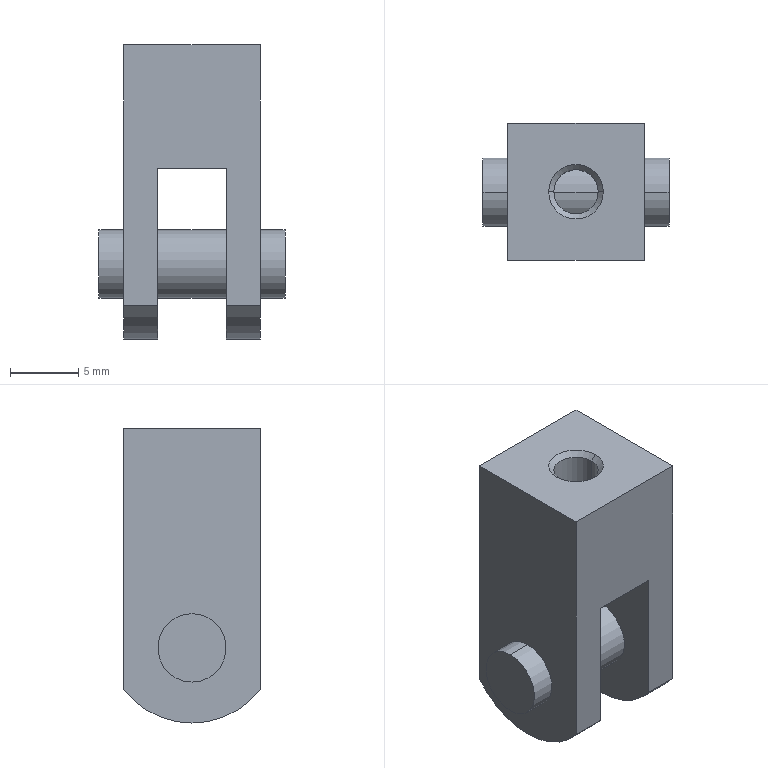Part | STEP file | Y_P010_Y-P010 | 1 solid | 22 faces | box 13.6 x 10 x 21.5 mm | volume 1582 mm3 | cylinder 10 | plane 10 | cone 2 | commonest cylinder face diameters 5 x6 3.24 x2 12.6 x2
STEP:
#1=CARTESIAN_POINT('',(6.8,0.,-18.5));
#2=VERTEX_POINT('',#1);
#3=CARTESIAN_POINT('',(6.8,0.,-13.5));
#4=VERTEX_POINT('',#3);
#5=CARTESIAN_POINT('',(6.8,0.,-16.));
#6=DIRECTION('',(1.,0.,0.));
#7=DIRECTION('',(0.,0.,-1.));
#8=AXIS2_PLACEMENT_3D('',#5,#6,#7);
#9=CIRCLE('',#8,2.5);
#10=EDGE_CURVE('',#2,#4,#9,.T.);
#11=ORIENTED_EDGE('',*,*,#10,.F.);
#12=CARTESIAN_POINT('',(5.,0.,-18.5));
#13=VERTEX_POINT('',#12);
#14=CARTESIAN_POINT('',(6.8,0.,-18.5));
#15=DIRECTION('',(-1.,0.,0.));
#16=VECTOR('',#15,1000.);
#17=LINE('',#14,#16);
#18=EDGE_CURVE('',#2,#13,#17,.T.);
#19=ORIENTED_EDGE('',*,*,#18,.T.);
#20=CARTESIAN_POINT('',(5.,0.,-13.5));
#21=VERTEX_POINT('',#20);
#22=CARTESIAN_POINT('',(5.,0.,-16.));
#23=DIRECTION('',(-1.,0.,0.));
#24=DIRECTION('',(0.,0.,-1.));
#25=AXIS2_PLACEMENT_3D('',#22,#23,#24);
#26=CIRCLE('',#25,2.5);
#27=EDGE_CURVE('',#21,#13,#26,.T.);
#28=ORIENTED_EDGE('',*,*,#27,.F.);
#29=CARTESIAN_POINT('',(6.8,0.,-13.5));
#30=DIRECTION('',(-1.,0.,0.));
#31=VECTOR('',#30,1000.);
#32=LINE('',#29,#31);
#33=EDGE_CURVE('',#4,#21,#32,.T.);
#34=ORIENTED_EDGE('',*,*,#33,.F.);
#35=EDGE_LOOP('',(#11,#19,#28,#34));
#36=FACE_OUTER_BOUND('',#35,.T.);
#37=CARTESIAN_POINT('',(6.8,0.,-16.));
#38=DIRECTION('',(-1.,0.,0.));
#39=DIRECTION('',(0.,0.,1.));
#40=AXIS2_PLACEMENT_3D('',#37,#38,#39);
#41=CYLINDRICAL_SURFACE('',#40,2.5);
#42=ADVANCED_FACE('',(#36),#41,.T.);
#43=CARTESIAN_POINT('',(-5.,0.,-13.5));
#44=VERTEX_POINT('',#43);
#45=CARTESIAN_POINT('',(-5.,0.,-18.5));
#46=VERTEX_POINT('',#45);
#47=CARTESIAN_POINT('',(-5.,0.,-16.));
#48=DIRECTION('',(-1.,0.,0.));
#49=DIRECTION('',(0.,0.,-1.));
#50=AXIS2_PLACEMENT_3D('',#47,#48,#49);
#51=CIRCLE('',#50,2.5);
#52=EDGE_CURVE('',#44,#46,#51,.T.);
#53=ORIENTED_EDGE('',*,*,#52,.T.);
#54=CARTESIAN_POINT('',(-6.8,0.,-18.5));
#55=VERTEX_POINT('',#54);
#56=CARTESIAN_POINT('',(6.8,0.,-18.5));
#57=DIRECTION('',(-1.,0.,0.));
#58=VECTOR('',#57,1000.);
#59=LINE('',#56,#58);
#60=EDGE_CURVE('',#46,#55,#59,.T.);
#61=ORIENTED_EDGE('',*,*,#60,.T.);
#62=CARTESIAN_POINT('',(-6.8,0.,-13.5));
#63=VERTEX_POINT('',#62);
#64=CARTESIAN_POINT('',(-6.8,0.,-16.));
#65=DIRECTION('',(1.,0.,0.));
#66=DIRECTION('',(0.,0.,-1.));
#67=AXIS2_PLACEMENT_3D('',#64,#65,#66);
#68=CIRCLE('',#67,2.5);
#69=EDGE_CURVE('',#55,#63,#68,.T.);
#70=ORIENTED_EDGE('',*,*,#69,.T.);
#71=CARTESIAN_POINT('',(6.8,0.,-13.5));
#72=DIRECTION('',(-1.,0.,0.));
#73=VECTOR('',#72,1000.);
#74=LINE('',#71,#73);
#75=EDGE_CURVE('',#44,#63,#74,.T.);
#76=ORIENTED_EDGE('',*,*,#75,.F.);
#77=EDGE_LOOP('',(#53,#61,#70,#76));
#78=FACE_OUTER_BOUND('',#77,.T.);
#79=CARTESIAN_POINT('',(6.8,0.,-16.));
#80=DIRECTION('',(-1.,0.,0.));
#81=DIRECTION('',(0.,0.,1.));
#82=AXIS2_PLACEMENT_3D('',#79,#80,#81);
#83=CYLINDRICAL_SURFACE('',#82,2.5);
#84=ADVANCED_FACE('',(#78),#83,.T.);
#85=CARTESIAN_POINT('',(2.5,0.,-13.5));
#86=VERTEX_POINT('',#85);
#87=CARTESIAN_POINT('',(2.5,0.,-18.5));
#88=VERTEX_POINT('',#87);
#89=CARTESIAN_POINT('',(2.5,0.,-16.));
#90=DIRECTION('',(-1.,0.,0.));
#91=DIRECTION('',(0.,0.,-1.));
#92=AXIS2_PLACEMENT_3D('',#89,#90,#91);
#93=CIRCLE('',#92,2.5);
#94=EDGE_CURVE('',#86,#88,#93,.T.);
#95=ORIENTED_EDGE('',*,*,#94,.T.);
#96=CARTESIAN_POINT('',(-2.5,0.,-18.5));
#97=VERTEX_POINT('',#96);
#98=CARTESIAN_POINT('',(6.8,0.,-18.5));
#99=DIRECTION('',(-1.,0.,0.));
#100=VECTOR('',#99,1000.);
#101=LINE('',#98,#100);
#102=EDGE_CURVE('',#88,#97,#101,.T.);
#103=ORIENTED_EDGE('',*,*,#102,.T.);
#104=CARTESIAN_POINT('',(-2.5,0.,-13.5));
#105=VERTEX_POINT('',#104);
#106=CARTESIAN_POINT('',(-2.5,0.,-16.));
#107=DIRECTION('',(-1.,0.,0.));
#108=DIRECTION('',(0.,0.,-1.));
#109=AXIS2_PLACEMENT_3D('',#106,#107,#108);
#110=CIRCLE('',#109,2.5);
#111=EDGE_CURVE('',#105,#97,#110,.T.);
#112=ORIENTED_EDGE('',*,*,#111,.F.);
#113=CARTESIAN_POINT('',(6.8,0.,-13.5));
#114=DIRECTION('',(-1.,0.,0.));
#115=VECTOR('',#114,1000.);
#116=LINE('',#113,#115);
#117=EDGE_CURVE('',#86,#105,#116,.T.);
#118=ORIENTED_EDGE('',*,*,#117,.F.);
#119=EDGE_LOOP('',(#95,#103,#112,#118));
#120=FACE_OUTER_BOUND('',#119,.T.);
#121=CARTESIAN_POINT('',(6.8,0.,-16.));
#122=DIRECTION('',(-1.,0.,0.));
#123=DIRECTION('',(0.,0.,1.));
#124=AXIS2_PLACEMENT_3D('',#121,#122,#123);
#125=CYLINDRICAL_SURFACE('',#124,2.5);
#126=ADVANCED_FACE('',(#120),#125,.T.);
#127=CARTESIAN_POINT('',(-1.62,0.,-9.));
#128=VERTEX_POINT('',#127);
#129=CARTESIAN_POINT('',(1.62,0.,-9.));
#130=VERTEX_POINT('',#129);
#131=CARTESIAN_POINT('',(0.,0.,-9.));
#132=DIRECTION('',(0.,0.,1.));
#133=DIRECTION('',(1.,0.,0.));
#134=AXIS2_PLACEMENT_3D('',#131,#132,#133);
#135=CIRCLE('',#134,1.62);
#136=EDGE_CURVE('',#128,#130,#135,.T.);
#137=ORIENTED_EDGE('',*,*,#136,.F.);
#138=CARTESIAN_POINT('',(-1.62,0.,-0.38));
#139=VERTEX_POINT('',#138);
#140=CARTESIAN_POINT('',(-1.62,0.,-9.));
#141=DIRECTION('',(0.,0.,1.));
#142=VECTOR('',#141,1000.);
#143=LINE('',#140,#142);
#144=EDGE_CURVE('',#128,#139,#143,.T.);
#145=ORIENTED_EDGE('',*,*,#144,.T.);
#146=CARTESIAN_POINT('',(1.62,0.,-0.38));
#147=VERTEX_POINT('',#146);
#148=CARTESIAN_POINT('',(0.,0.,-0.38));
#149=DIRECTION('',(0.,0.,1.));
#150=DIRECTION('',(1.,0.,0.));
#151=AXIS2_PLACEMENT_3D('',#148,#149,#150);
#152=CIRCLE('',#151,1.62);
#153=EDGE_CURVE('',#139,#147,#152,.T.);
#154=ORIENTED_EDGE('',*,*,#153,.T.);
#155=CARTESIAN_POINT('',(1.62,0.,-9.));
#156=DIRECTION('',(0.,0.,1.));
#157=VECTOR('',#156,1000.);
#158=LINE('',#155,#157);
#159=EDGE_CURVE('',#130,#147,#158,.T.);
#160=ORIENTED_EDGE('',*,*,#159,.F.);
#161=EDGE_LOOP('',(#137,#145,#154,#160));
#162=FACE_OUTER_BOUND('',#161,.T.);
#163=CARTESIAN_POINT('',(0.,0.,-9.));
#164=DIRECTION('',(0.,0.,1.));
#165=DIRECTION('',(1.,0.,0.));
#166=AXIS2_PLACEMENT_3D('',#163,#164,#165);
#167=CYLINDRICAL_SURFACE('',#166,1.62);
#168=ADVANCED_FACE('',(#162),#167,.F.);
#169=ORIENTED_EDGE('',*,*,#153,.F.);
#170=CARTESIAN_POINT('',(-2.,0.,0.));
#171=VERTEX_POINT('',#170);
#172=CARTESIAN_POINT('',(-1.62,0.,-0.38));
#173=DIRECTION('',(-0.7071,0.,0.7071));
#174=VECTOR('',#173,1000.);
#175=LINE('',#172,#174);
#176=EDGE_CURVE('',#139,#171,#175,.T.);
#177=ORIENTED_EDGE('',*,*,#176,.T.);
#178=CARTESIAN_POINT('',(2.,0.,0.));
#179=VERTEX_POINT('',#178);
#180=CARTESIAN_POINT('',(0.,0.,0.));
#181=DIRECTION('',(0.,0.,1.));
#182=DIRECTION('',(-1.,0.,0.));
#183=AXIS2_PLACEMENT_3D('',#180,#181,#182);
#184=CIRCLE('',#183,2.);
#185=EDGE_CURVE('',#171,#179,#184,.T.);
#186=ORIENTED_EDGE('',*,*,#185,.T.);
#187=CARTESIAN_POINT('',(1.62,0.,-0.38));
#188=DIRECTION('',(0.7071,0.,0.7071));
#189=VECTOR('',#188,1000.);
#190=LINE('',#187,#189);
#191=EDGE_CURVE('',#147,#179,#190,.T.);
#192=ORIENTED_EDGE('',*,*,#191,.F.);
#193=EDGE_LOOP('',(#169,#177,#186,#192));
#194=FACE_OUTER_BOUND('',#193,.T.);
#195=CARTESIAN_POINT('',(0.,0.,-0.38));
#196=DIRECTION('',(0.,0.,1.));
#197=DIRECTION('',(1.,0.,0.));
#198=AXIS2_PLACEMENT_3D('',#195,#196,#197);
#199=CONICAL_SURFACE('',#198,1.62,0.7854);
#200=ADVANCED_FACE('',(#194),#199,.F.);
#201=CARTESIAN_POINT('',(5.,5.,0.));
#202=VERTEX_POINT('',#201);
#203=CARTESIAN_POINT('',(5.,-5.,0.));
#204=VERTEX_POINT('',#203);
#205=CARTESIAN_POINT('',(5.,5.,0.));
#206=DIRECTION('',(0.,-1.,0.));
#207=VECTOR('',#206,1000.);
#208=LINE('',#205,#207);
#209=EDGE_CURVE('',#202,#204,#208,.T.);
#210=ORIENTED_EDGE('',*,*,#209,.T.);
#211=CARTESIAN_POINT('',(5.,-5.,-19.033));
#212=VERTEX_POINT('',#211);
#213=CARTESIAN_POINT('',(5.,-5.,0.));
#214=DIRECTION('',(0.,0.,-1.));
#215=VECTOR('',#214,1000.);
#216=LINE('',#213,#215);
#217=EDGE_CURVE('',#204,#212,#216,.T.);
#218=ORIENTED_EDGE('',*,*,#217,.T.);
#219=CARTESIAN_POINT('',(5.,5.,-19.033));
#220=VERTEX_POINT('',#219);
#221=CARTESIAN_POINT('',(5.,0.,-15.2));
#222=DIRECTION('',(1.,0.,0.));
#223=DIRECTION('',(0.,0.,-1.));
#224=AXIS2_PLACEMENT_3D('',#221,#222,#223);
#225=CIRCLE('',#224,6.3);
#226=EDGE_CURVE('',#212,#220,#225,.T.);
#227=ORIENTED_EDGE('',*,*,#226,.T.);
#228=CARTESIAN_POINT('',(5.,5.,-19.033));
#229=DIRECTION('',(0.,0.,1.));
#230=VECTOR('',#229,1000.);
#231=LINE('',#228,#230);
#232=EDGE_CURVE('',#220,#202,#231,.T.);
#233=ORIENTED_EDGE('',*,*,#232,.T.);
#234=EDGE_LOOP('',(#210,#218,#227,#233));
#235=FACE_OUTER_BOUND('',#234,.T.);
#236=ORIENTED_EDGE('',*,*,#27,.T.);
#237=CARTESIAN_POINT('',(5.,0.,-16.));
#238=DIRECTION('',(-1.,0.,0.));
#239=DIRECTION('',(0.,0.,-1.));
#240=AXIS2_PLACEMENT_3D('',#237,#238,#239);
#241=CIRCLE('',#240,2.5);
#242=EDGE_CURVE('',#13,#21,#241,.T.);
#243=ORIENTED_EDGE('',*,*,#242,.T.);
#244=EDGE_LOOP('',(#236,#243));
#245=FACE_BOUND('',#244,.T.);
#246=CARTESIAN_POINT('',(5.,0.,-15.2));
#247=DIRECTION('',(1.,0.,0.));
#248=DIRECTION('',(0.,0.,-1.));
#249=AXIS2_PLACEMENT_3D('',#246,#247,#248);
#250=PLANE('',#249);
#251=ADVANCED_FACE('',(#235,#245),#250,.T.);
#252=CARTESIAN_POINT('',(-5.,5.,0.));
#253=VERTEX_POINT('',#252);
#254=CARTESIAN_POINT('',(-5.,-5.,0.));
#255=VERTEX_POINT('',#254);
#256=CARTESIAN_POINT('',(-5.,5.,0.));
#257=DIRECTION('',(0.,-1.,0.));
#258=VECTOR('',#257,1000.);
#259=LINE('',#256,#258);
#260=EDGE_CURVE('',#253,#255,#259,.T.);
#261=ORIENTED_EDGE('',*,*,#260,.F.);
#262=CARTESIAN_POINT('',(-5.,5.,-19.033));
#263=VERTEX_POINT('',#262);
#264=CARTESIAN_POINT('',(-5.,5.,-19.033));
#265=DIRECTION('',(0.,0.,1.));
#266=VECTOR('',#265,1000.);
#267=LINE('',#264,#266);
#268=EDGE_CURVE('',#263,#253,#267,.T.);
#269=ORIENTED_EDGE('',*,*,#268,.F.);
#270=CARTESIAN_POINT('',(-5.,-5.,-19.033));
#271=VERTEX_POINT('',#270);
#272=CARTESIAN_POINT('',(-5.,0.,-15.2));
#273=DIRECTION('',(1.,0.,0.));
#274=DIRECTION('',(0.,0.,-1.));
#275=AXIS2_PLACEMENT_3D('',#272,#273,#274);
#276=CIRCLE('',#275,6.3);
#277=EDGE_CURVE('',#271,#263,#276,.T.);
#278=ORIENTED_EDGE('',*,*,#277,.F.);
#279=CARTESIAN_POINT('',(-5.,-5.,0.));
#280=DIRECTION('',(0.,0.,-1.));
#281=VECTOR('',#280,1000.);
#282=LINE('',#279,#281);
#283=EDGE_CURVE('',#255,#271,#282,.T.);
#284=ORIENTED_EDGE('',*,*,#283,.F.);
#285=EDGE_LOOP('',(#261,#269,#278,#284));
#286=FACE_OUTER_BOUND('',#285,.T.);
#287=ORIENTED_EDGE('',*,*,#52,.F.);
#288=CARTESIAN_POINT('',(-5.,0.,-16.));
#289=DIRECTION('',(-1.,0.,0.));
#290=DIRECTION('',(0.,0.,-1.));
#291=AXIS2_PLACEMENT_3D('',#288,#289,#290);
#292=CIRCLE('',#291,2.5);
#293=EDGE_CURVE('',#46,#44,#292,.T.);
#294=ORIENTED_EDGE('',*,*,#293,.F.);
#295=EDGE_LOOP('',(#287,#294));
#296=FACE_BOUND('',#295,.T.);
#297=CARTESIAN_POINT('',(-5.,0.,-15.2));
#298=DIRECTION('',(1.,0.,0.));
#299=DIRECTION('',(0.,0.,-1.));
#300=AXIS2_PLACEMENT_3D('',#297,#298,#299);
#301=PLANE('',#300);
#302=ADVANCED_FACE('',(#286,#296),#301,.F.);
#303=CARTESIAN_POINT('',(-2.5,-5.,-9.));
#304=VERTEX_POINT('',#303);
#305=CARTESIAN_POINT('',(-2.5,-5.,-19.033));
#306=VERTEX_POINT('',#305);
#307=CARTESIAN_POINT('',(-2.5,-5.,0.));
#308=DIRECTION('',(0.,0.,-1.));
#309=VECTOR('',#308,1000.);
#310=LINE('',#307,#309);
#311=EDGE_CURVE('',#304,#306,#310,.T.);
#312=ORIENTED_EDGE('',*,*,#311,.T.);
#313=CARTESIAN_POINT('',(-2.5,5.,-19.033));
#314=VERTEX_POINT('',#313);
#315=CARTESIAN_POINT('',(-2.5,0.,-15.2));
#316=DIRECTION('',(1.,0.,0.));
#317=DIRECTION('',(0.,0.,-1.));
#318=AXIS2_PLACEMENT_3D('',#315,#316,#317);
#319=CIRCLE('',#318,6.3);
#320=EDGE_CURVE('',#306,#314,#319,.T.);
#321=ORIENTED_EDGE('',*,*,#320,.T.);
#322=CARTESIAN_POINT('',(-2.5,5.,-9.));
#323=VERTEX_POINT('',#322);
#324=CARTESIAN_POINT('',(-2.5,5.,-19.033));
#325=DIRECTION('',(0.,0.,1.));
#326=VECTOR('',#325,1000.);
#327=LINE('',#324,#326);
#328=EDGE_CURVE('',#314,#323,#327,.T.);
#329=ORIENTED_EDGE('',*,*,#328,.T.);
#330=CARTESIAN_POINT('',(-2.5,5.01,-9.));
#331=DIRECTION('',(0.,-1.,0.));
#332=VECTOR('',#331,1000.);
#333=LINE('',#330,#332);
#334=EDGE_CURVE('',#323,#304,#333,.T.);
#335=ORIENTED_EDGE('',*,*,#334,.T.);
#336=EDGE_LOOP('',(#312,#321,#329,#335));
#337=FACE_OUTER_BOUND('',#336,.T.);
#338=ORIENTED_EDGE('',*,*,#111,.T.);
#339=CARTESIAN_POINT('',(-2.5,0.,-16.));
#340=DIRECTION('',(-1.,0.,0.));
#341=DIRECTION('',(0.,0.,-1.));
#342=AXIS2_PLACEMENT_3D('',#339,#340,#341);
#343=CIRCLE('',#342,2.5);
#344=EDGE_CURVE('',#97,#105,#343,.T.);
#345=ORIENTED_EDGE('',*,*,#344,.T.);
#346=EDGE_LOOP('',(#338,#345));
#347=FACE_BOUND('',#346,.T.);
#348=CARTESIAN_POINT('',(-2.5,-5.01,-9.));
#349=DIRECTION('',(1.,0.,0.));
#350=DIRECTION('',(0.,0.,-1.));
#351=AXIS2_PLACEMENT_3D('',#348,#349,#350);
#352=PLANE('',#351);
#353=ADVANCED_FACE('',(#337,#347),#352,.T.);
#354=CARTESIAN_POINT('',(2.5,5.,-9.));
#355=VERTEX_POINT('',#354);
#356=CARTESIAN_POINT('',(2.5,-5.,-9.));
#357=VERTEX_POINT('',#356);
#358=CARTESIAN_POINT('',(2.5,5.01,-9.));
#359=DIRECTION('',(0.,-1.,0.));
#360=VECTOR('',#359,1000.);
#361=LINE('',#358,#360);
#362=EDGE_CURVE('',#355,#357,#361,.T.);
#363=ORIENTED_EDGE('',*,*,#362,.F.);
#364=CARTESIAN_POINT('',(2.5,5.,-19.033));
#365=VERTEX_POINT('',#364);
#366=CARTESIAN_POINT('',(2.5,5.,-19.033));
#367=DIRECTION('',(0.,0.,1.));
#368=VECTOR('',#367,1000.);
#369=LINE('',#366,#368);
#370=EDGE_CURVE('',#365,#355,#369,.T.);
#371=ORIENTED_EDGE('',*,*,#370,.F.);
#372=CARTESIAN_POINT('',(2.5,-5.,-19.033));
#373=VERTEX_POINT('',#372);
#374=CARTESIAN_POINT('',(2.5,0.,-15.2));
#375=DIRECTION('',(1.,0.,0.));
#376=DIRECTION('',(0.,0.,-1.));
#377=AXIS2_PLACEMENT_3D('',#374,#375,#376);
#378=CIRCLE('',#377,6.3);
#379=EDGE_CURVE('',#373,#365,#378,.T.);
#380=ORIENTED_EDGE('',*,*,#379,.F.);
#381=CARTESIAN_POINT('',(2.5,-5.,0.));
#382=DIRECTION('',(0.,0.,-1.));
#383=VECTOR('',#382,1000.);
#384=LINE('',#381,#383);
#385=EDGE_CURVE('',#357,#373,#384,.T.);
#386=ORIENTED_EDGE('',*,*,#385,.F.);
#387=EDGE_LOOP('',(#363,#371,#380,#386));
#388=FACE_OUTER_BOUND('',#387,.T.);
#389=ORIENTED_EDGE('',*,*,#94,.F.);
#390=CARTESIAN_POINT('',(2.5,0.,-16.));
#391=DIRECTION('',(-1.,0.,0.));
#392=DIRECTION('',(0.,0.,-1.));
#393=AXIS2_PLACEMENT_3D('',#390,#391,#392);
#394=CIRCLE('',#393,2.5);
#395=EDGE_CURVE('',#88,#86,#394,.T.);
#396=ORIENTED_EDGE('',*,*,#395,.F.);
#397=EDGE_LOOP('',(#389,#396));
#398=FACE_BOUND('',#397,.T.);
#399=CARTESIAN_POINT('',(2.5,-5.01,-9.));
#400=DIRECTION('',(1.,0.,0.));
#401=DIRECTION('',(0.,0.,-1.));
#402=AXIS2_PLACEMENT_3D('',#399,#400,#401);
#403=PLANE('',#402);
#404=ADVANCED_FACE('',(#388,#398),#403,.F.);
#405=CARTESIAN_POINT('',(5.,5.,0.));
#406=DIRECTION('',(-1.,0.,0.));
#407=VECTOR('',#406,1000.);
#408=LINE('',#405,#407);
#409=EDGE_CURVE('',#202,#253,#408,.T.);
#410=ORIENTED_EDGE('',*,*,#409,.T.);
#411=ORIENTED_EDGE('',*,*,#260,.T.);
#412=CARTESIAN_POINT('',(5.,-5.,0.));
#413=DIRECTION('',(-1.,0.,0.));
#414=VECTOR('',#413,1000.);
#415=LINE('',#412,#414);
#416=EDGE_CURVE('',#204,#255,#415,.T.);
#417=ORIENTED_EDGE('',*,*,#416,.F.);
#418=ORIENTED_EDGE('',*,*,#209,.F.);
#419=EDGE_LOOP('',(#410,#411,#417,#418));
#420=FACE_OUTER_BOUND('',#419,.T.);
#421=CARTESIAN_POINT('',(0.,0.,0.));
#422=DIRECTION('',(0.,0.,1.));
#423=DIRECTION('',(-1.,0.,0.));
#424=AXIS2_PLACEMENT_3D('',#421,#422,#423);
#425=CIRCLE('',#424,2.);
#426=EDGE_CURVE('',#179,#171,#425,.T.);
#427=ORIENTED_EDGE('',*,*,#426,.F.);
#428=ORIENTED_EDGE('',*,*,#185,.F.);
#429=EDGE_LOOP('',(#427,#428));
#430=FACE_BOUND('',#429,.T.);
#431=CARTESIAN_POINT('',(5.,5.,0.));
#432=DIRECTION('',(0.,0.,-1.));
#433=DIRECTION('',(-1.,0.,0.));
#434=AXIS2_PLACEMENT_3D('',#431,#432,#433);
#435=PLANE('',#434);
#436=ADVANCED_FACE('',(#420,#430),#435,.F.);
#437=ORIENTED_EDGE('',*,*,#334,.F.);
#438=CARTESIAN_POINT('',(5.,5.,-9.));
#439=DIRECTION('',(-1.,0.,0.));
#440=VECTOR('',#439,1000.);
#441=LINE('',#438,#440);
#442=EDGE_CURVE('',#355,#323,#441,.T.);
#443=ORIENTED_EDGE('',*,*,#442,.F.);
#444=ORIENTED_EDGE('',*,*,#362,.T.);
#445=CARTESIAN_POINT('',(5.,-5.,-9.));
#446=DIRECTION('',(1.,0.,0.));
#447=VECTOR('',#446,1000.);
#448=LINE('',#445,#447);
#449=EDGE_CURVE('',#304,#357,#448,.T.);
#450=ORIENTED_EDGE('',*,*,#449,.F.);
#451=EDGE_LOOP('',(#437,#443,#444,#450));
#452=FACE_OUTER_BOUND('',#451,.T.);
#453=CARTESIAN_POINT('',(0.,0.,-9.));
#454=DIRECTION('',(0.,0.,1.));
#455=DIRECTION('',(1.,0.,0.));
#456=AXIS2_PLACEMENT_3D('',#453,#454,#455);
#457=CIRCLE('',#456,1.62);
#458=EDGE_CURVE('',#130,#128,#457,.T.);
#459=ORIENTED_EDGE('',*,*,#458,.T.);
#460=ORIENTED_EDGE('',*,*,#136,.T.);
#461=EDGE_LOOP('',(#459,#460));
#462=FACE_BOUND('',#461,.T.);
#463=CARTESIAN_POINT('',(-2.5,5.01,-9.));
#464=DIRECTION('',(0.,0.,1.));
#465=DIRECTION('',(1.,0.,0.));
#466=AXIS2_PLACEMENT_3D('',#463,#464,#465);
#467=PLANE('',#466);
#468=ADVANCED_FACE('',(#452,#462),#467,.F.);
#469=ORIENTED_EDGE('',*,*,#311,.F.);
#470=ORIENTED_EDGE('',*,*,#449,.T.);
#471=ORIENTED_EDGE('',*,*,#385,.T.);
#472=CARTESIAN_POINT('',(5.,-5.,-19.033));
#473=DIRECTION('',(-1.,0.,0.));
#474=VECTOR('',#473,1000.);
#475=LINE('',#472,#474);
#476=EDGE_CURVE('',#212,#373,#475,.T.);
#477=ORIENTED_EDGE('',*,*,#476,.F.);
#478=ORIENTED_EDGE('',*,*,#217,.F.);
#479=ORIENTED_EDGE('',*,*,#416,.T.);
#480=ORIENTED_EDGE('',*,*,#283,.T.);
#481=CARTESIAN_POINT('',(5.,-5.,-19.033));
#482=DIRECTION('',(-1.,0.,0.));
#483=VECTOR('',#482,1000.);
#484=LINE('',#481,#483);
#485=EDGE_CURVE('',#306,#271,#484,.T.);
#486=ORIENTED_EDGE('',*,*,#485,.F.);
#487=EDGE_LOOP('',(#469,#470,#471,#477,#478,#479,#480,#486));
#488=FACE_OUTER_BOUND('',#487,.T.);
#489=CARTESIAN_POINT('',(5.,-5.,0.));
#490=DIRECTION('',(0.,1.,0.));
#491=DIRECTION('',(0.,0.,1.));
#492=AXIS2_PLACEMENT_3D('',#489,#490,#491);
#493=PLANE('',#492);
#494=ADVANCED_FACE('',(#488),#493,.F.);
#495=ORIENTED_EDGE('',*,*,#320,.F.);
#496=ORIENTED_EDGE('',*,*,#485,.T.);
#497=ORIENTED_EDGE('',*,*,#277,.T.);
#498=CARTESIAN_POINT('',(5.,5.,-19.033));
#499=DIRECTION('',(-1.,0.,0.));
#500=VECTOR('',#499,1000.);
#501=LINE('',#498,#500);
#502=EDGE_CURVE('',#314,#263,#501,.T.);
#503=ORIENTED_EDGE('',*,*,#502,.F.);
#504=EDGE_LOOP('',(#495,#496,#497,#503));
#505=FACE_OUTER_BOUND('',#504,.T.);
#506=CARTESIAN_POINT('',(5.,0.,-15.2));
#507=DIRECTION('',(-1.,0.,0.));
#508=DIRECTION('',(0.,0.,1.));
#509=AXIS2_PLACEMENT_3D('',#506,#507,#508);
#510=CYLINDRICAL_SURFACE('',#509,6.3);
#511=ADVANCED_FACE('',(#505),#510,.T.);
#512=ORIENTED_EDGE('',*,*,#328,.F.);
#513=ORIENTED_EDGE('',*,*,#502,.T.);
#514=ORIENTED_EDGE('',*,*,#268,.T.);
#515=ORIENTED_EDGE('',*,*,#409,.F.);
#516=ORIENTED_EDGE('',*,*,#232,.F.);
#517=CARTESIAN_POINT('',(5.,5.,-19.033));
#518=DIRECTION('',(-1.,0.,0.));
#519=VECTOR('',#518,1000.);
#520=LINE('',#517,#519);
#521=EDGE_CURVE('',#220,#365,#520,.T.);
#522=ORIENTED_EDGE('',*,*,#521,.T.);
#523=ORIENTED_EDGE('',*,*,#370,.T.);
#524=ORIENTED_EDGE('',*,*,#442,.T.);
#525=EDGE_LOOP('',(#512,#513,#514,#515,#516,#522,#523,#524));
#526=FACE_OUTER_BOUND('',#525,.T.);
#527=CARTESIAN_POINT('',(5.,5.,-19.033));
#528=DIRECTION('',(0.,-1.,0.));
#529=DIRECTION('',(0.,0.,-1.));
#530=AXIS2_PLACEMENT_3D('',#527,#528,#529);
#531=PLANE('',#530);
#532=ADVANCED_FACE('',(#526),#531,.F.);
#533=ORIENTED_EDGE('',*,*,#476,.T.);
#534=ORIENTED_EDGE('',*,*,#379,.T.);
#535=ORIENTED_EDGE('',*,*,#521,.F.);
#536=ORIENTED_EDGE('',*,*,#226,.F.);
#537=EDGE_LOOP('',(#533,#534,#535,#536));
#538=FACE_OUTER_BOUND('',#537,.T.);
#539=CARTESIAN_POINT('',(5.,0.,-15.2));
#540=DIRECTION('',(-1.,0.,0.));
#541=DIRECTION('',(0.,0.,1.));
#542=AXIS2_PLACEMENT_3D('',#539,#540,#541);
#543=CYLINDRICAL_SURFACE('',#542,6.3);
#544=ADVANCED_FACE('',(#538),#543,.T.);
#545=ORIENTED_EDGE('',*,*,#176,.F.);
#546=CARTESIAN_POINT('',(0.,0.,-0.38));
#547=DIRECTION('',(0.,0.,1.));
#548=DIRECTION('',(1.,0.,0.));
#549=AXIS2_PLACEMENT_3D('',#546,#547,#548);
#550=CIRCLE('',#549,1.62);
#551=EDGE_CURVE('',#147,#139,#550,.T.);
#552=ORIENTED_EDGE('',*,*,#551,.F.);
#553=ORIENTED_EDGE('',*,*,#191,.T.);
#554=ORIENTED_EDGE('',*,*,#426,.T.);
#555=EDGE_LOOP('',(#545,#552,#553,#554));
#556=FACE_OUTER_BOUND('',#555,.T.);
#557=CARTESIAN_POINT('',(0.,0.,-0.38));
#558=DIRECTION('',(0.,0.,1.));
#559=DIRECTION('',(1.,0.,0.));
#560=AXIS2_PLACEMENT_3D('',#557,#558,#559);
#561=CONICAL_SURFACE('',#560,1.62,0.7854);
#562=ADVANCED_FACE('',(#556),#561,.F.);
#563=ORIENTED_EDGE('',*,*,#144,.F.);
#564=ORIENTED_EDGE('',*,*,#458,.F.);
#565=ORIENTED_EDGE('',*,*,#159,.T.);
#566=ORIENTED_EDGE('',*,*,#551,.T.);
#567=EDGE_LOOP('',(#563,#564,#565,#566));
#568=FACE_OUTER_BOUND('',#567,.T.);
#569=CARTESIAN_POINT('',(0.,0.,-9.));
#570=DIRECTION('',(0.,0.,1.));
#571=DIRECTION('',(1.,0.,0.));
#572=AXIS2_PLACEMENT_3D('',#569,#570,#571);
#573=CYLINDRICAL_SURFACE('',#572,1.62);
#574=ADVANCED_FACE('',(#568),#573,.F.);
#575=ORIENTED_EDGE('',*,*,#102,.F.);
#576=ORIENTED_EDGE('',*,*,#395,.T.);
#577=ORIENTED_EDGE('',*,*,#117,.T.);
#578=ORIENTED_EDGE('',*,*,#344,.F.);
#579=EDGE_LOOP('',(#575,#576,#577,#578));
#580=FACE_OUTER_BOUND('',#579,.T.);
#581=CARTESIAN_POINT('',(6.8,0.,-16.));
#582=DIRECTION('',(-1.,0.,0.));
#583=DIRECTION('',(0.,0.,1.));
#584=AXIS2_PLACEMENT_3D('',#581,#582,#583);
#585=CYLINDRICAL_SURFACE('',#584,2.5);
#586=ADVANCED_FACE('',(#580),#585,.T.);
#587=CARTESIAN_POINT('',(-6.8,0.,-16.));
#588=DIRECTION('',(1.,0.,0.));
#589=DIRECTION('',(0.,0.,-1.));
#590=AXIS2_PLACEMENT_3D('',#587,#588,#589);
#591=CIRCLE('',#590,2.5);
#592=EDGE_CURVE('',#63,#55,#591,.T.);
#593=ORIENTED_EDGE('',*,*,#592,.F.);
#594=ORIENTED_EDGE('',*,*,#69,.F.);
#595=EDGE_LOOP('',(#593,#594));
#596=FACE_OUTER_BOUND('',#595,.T.);
#597=CARTESIAN_POINT('',(-6.8,0.,-16.));
#598=DIRECTION('',(1.,0.,0.));
#599=DIRECTION('',(0.,0.,-1.));
#600=AXIS2_PLACEMENT_3D('',#597,#598,#599);
#601=PLANE('',#600);
#602=ADVANCED_FACE('',(#596),#601,.F.);
#603=ORIENTED_EDGE('',*,*,#60,.F.);
#604=ORIENTED_EDGE('',*,*,#293,.T.);
#605=ORIENTED_EDGE('',*,*,#75,.T.);
#606=ORIENTED_EDGE('',*,*,#592,.T.);
#607=EDGE_LOOP('',(#603,#604,#605,#606));
#608=FACE_OUTER_BOUND('',#607,.T.);
#609=CARTESIAN_POINT('',(6.8,0.,-16.));
#610=DIRECTION('',(-1.,0.,0.));
#611=DIRECTION('',(0.,0.,1.));
#612=AXIS2_PLACEMENT_3D('',#609,#610,#611);
#613=CYLINDRICAL_SURFACE('',#612,2.5);
#614=ADVANCED_FACE('',(#608),#613,.T.);
#615=ORIENTED_EDGE('',*,*,#18,.F.);
#616=CARTESIAN_POINT('',(6.8,0.,-16.));
#617=DIRECTION('',(1.,0.,0.));
#618=DIRECTION('',(0.,0.,-1.));
#619=AXIS2_PLACEMENT_3D('',#616,#617,#618);
#620=CIRCLE('',#619,2.5);
#621=EDGE_CURVE('',#4,#2,#620,.T.);
#622=ORIENTED_EDGE('',*,*,#621,.F.);
#623=ORIENTED_EDGE('',*,*,#33,.T.);
#624=ORIENTED_EDGE('',*,*,#242,.F.);
#625=EDGE_LOOP('',(#615,#622,#623,#624));
#626=FACE_OUTER_BOUND('',#625,.T.);
#627=CARTESIAN_POINT('',(6.8,0.,-16.));
#628=DIRECTION('',(-1.,0.,0.));
#629=DIRECTION('',(0.,0.,1.));
#630=AXIS2_PLACEMENT_3D('',#627,#628,#629);
#631=CYLINDRICAL_SURFACE('',#630,2.5);
#632=ADVANCED_FACE('',(#626),#631,.T.);
#633=ORIENTED_EDGE('',*,*,#621,.T.);
#634=ORIENTED_EDGE('',*,*,#10,.T.);
#635=EDGE_LOOP('',(#633,#634));
#636=FACE_OUTER_BOUND('',#635,.T.);
#637=CARTESIAN_POINT('',(6.8,0.,-16.));
#638=DIRECTION('',(1.,0.,0.));
#639=DIRECTION('',(0.,0.,-1.));
#640=AXIS2_PLACEMENT_3D('',#637,#638,#639);
#641=PLANE('',#640);
#642=ADVANCED_FACE('',(#636),#641,.T.);
#643=CLOSED_SHELL('',(#42,#84,#126,#168,#200,#251,#302,#353,#404,#436,#468,#494,#511,#532,#544,#562,#574,#586,#602,#614,#632,#642));
#644=MANIFOLD_SOLID_BREP('',#643);
#645=CARTESIAN_POINT('',(0.,0.,0.));
#646=DIRECTION('',(0.,0.,1.));
#647=DIRECTION('',(1.,0.,0.));
#648=AXIS2_PLACEMENT_3D('',#645,#646,#647);
#649=(LENGTH_UNIT()NAMED_UNIT(*)SI_UNIT(.MILLI.,.METRE.));
#650=UNCERTAINTY_MEASURE_WITH_UNIT(LENGTH_MEASURE(0.00001),#649,'','');
#651=(NAMED_UNIT(*)PLANE_ANGLE_UNIT()SI_UNIT($,.RADIAN.));
#652=(NAMED_UNIT(*)SI_UNIT($,.STERADIAN.)SOLID_ANGLE_UNIT());
#653=(GEOMETRIC_REPRESENTATION_CONTEXT(3)GLOBAL_UNCERTAINTY_ASSIGNED_CONTEXT((#650))GLOBAL_UNIT_ASSIGNED_CONTEXT((#649,#651,#652))REPRESENTATION_CONTEXT('',''));
#654=ADVANCED_BREP_SHAPE_REPRESENTATION('',(#644,#648),#653);